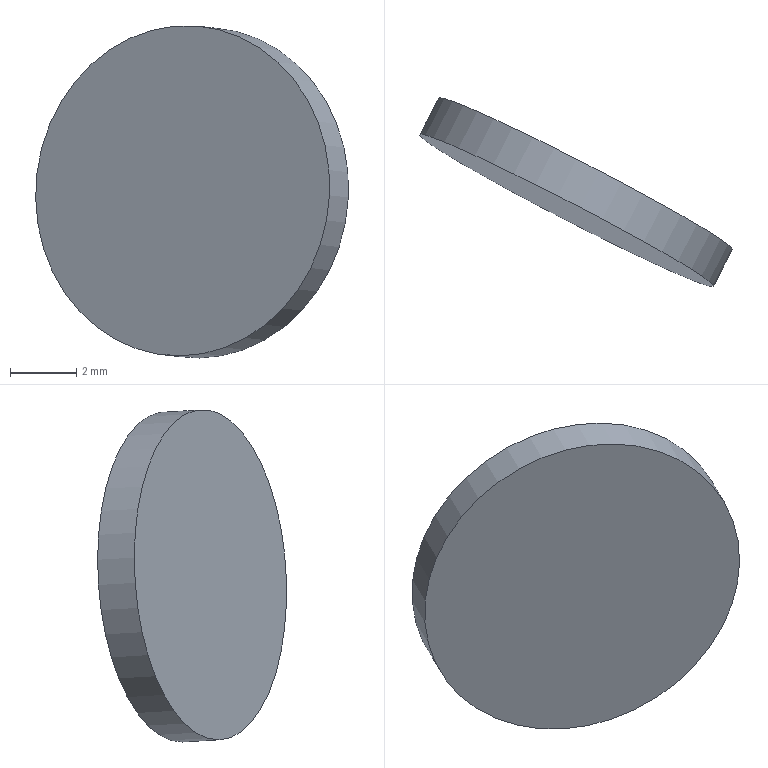Part | STEP file | gslz 2016.10.28-13_id54_x_t | 1 solid | 3 faces | box 9.464 x 5.714 x 10.052 mm | volume 98.175 mm3 | plane 2 | cylinder 1 | commonest cylinder face diameters 10 x1
STEP:
#1=CARTESIAN_POINT('',(0.,0.,0.));
#2=DIRECTION('',(0.,0.,1.));
#3=DIRECTION('',(1.,0.,0.));
#4=AXIS2_PLACEMENT_3D('',#1,#2,#3);
#5=CARTESIAN_POINT('',(875.587,-212.928,-20.691));
#6=VERTEX_POINT('',#5);
#7=CARTESIAN_POINT('',(875.855,-213.36,-25.665));
#8=DIRECTION('',(0.4575,0.8877,-0.05248));
#9=DIRECTION('',(-0.05363,0.08645,0.9948));
#10=AXIS2_PLACEMENT_3D('',#7,#8,#9);
#11=CIRCLE('',#10,5.);
#12=CARTESIAN_POINT('',(876.427,-212.25,-25.731));
#13=DIRECTION('',(-0.4575,-0.8877,0.05248));
#14=DIRECTION('',(0.8889,-0.4581,0.));
#15=AXIS2_PLACEMENT_3D('',#12,#13,#14);
#16=CYLINDRICAL_SURFACE('',#15,5.);
#17=CARTESIAN_POINT('',(7.941,1.25));
#18=DIRECTION('',(-1.,0.));
#19=VECTOR('',#18,1.);
#20=LINE('',#17,#19);
#21=(GEOMETRIC_REPRESENTATION_CONTEXT(2)PARAMETRIC_REPRESENTATION_CONTEXT()REPRESENTATION_CONTEXT('',''));
#22=DEFINITIONAL_REPRESENTATION('',(#20),#21);
#23=PCURVE('',#16,#22);
#24=CARTESIAN_POINT('',(875.855,-213.36,-25.665));
#25=DIRECTION('',(0.4575,0.8877,-0.05248));
#26=DIRECTION('',(-0.8889,0.4581,0.));
#27=AXIS2_PLACEMENT_3D('',#24,#25,#26);
#28=PLANE('',#27);
#29=CARTESIAN_POINT('',(0.,0.));
#30=DIRECTION('',(0.08728,0.9962));
#31=AXIS2_PLACEMENT_2D('',#29,#30);
#32=CIRCLE('',#31,5.);
#33=(GEOMETRIC_REPRESENTATION_CONTEXT(2)PARAMETRIC_REPRESENTATION_CONTEXT()REPRESENTATION_CONTEXT('',''));
#34=DEFINITIONAL_REPRESENTATION('',(#32),#33);
#35=PCURVE('',#28,#34);
#36=SURFACE_CURVE('',#11,(#23,#35),.PCURVE_S1.);
#37=EDGE_CURVE('',#6,#6,#36,.T.);
#38=ORIENTED_EDGE('',*,*,#37,.T.);
#39=CARTESIAN_POINT('',(876.159,-211.818,-20.757));
#40=VERTEX_POINT('',#39);
#41=CARTESIAN_POINT('',(876.159,-211.818,-20.757));
#42=CARTESIAN_POINT('',(875.587,-212.928,-20.691));
#43=B_SPLINE_CURVE_WITH_KNOTS('',1,(#41,#42),.UNSPECIFIED.,.F.,.F.,(2,2),(0.,1.25),.PIECEWISE_BEZIER_KNOTS.);
#44=CARTESIAN_POINT('',(1.658,0.));
#45=DIRECTION('',(0.,1.));
#46=VECTOR('',#45,1.);
#47=LINE('',#44,#46);
#48=(GEOMETRIC_REPRESENTATION_CONTEXT(2)PARAMETRIC_REPRESENTATION_CONTEXT()REPRESENTATION_CONTEXT('',''));
#49=DEFINITIONAL_REPRESENTATION('',(#47),#48);
#50=PCURVE('',#16,#49);
#51=CARTESIAN_POINT('',(7.941,0.));
#52=DIRECTION('',(0.,1.));
#53=VECTOR('',#52,1.);
#54=LINE('',#51,#53);
#55=(GEOMETRIC_REPRESENTATION_CONTEXT(2)PARAMETRIC_REPRESENTATION_CONTEXT()REPRESENTATION_CONTEXT('',''));
#56=DEFINITIONAL_REPRESENTATION('',(#54),#55);
#57=PCURVE('',#16,#56);
#58=SEAM_CURVE('',#43,(#50,#57),.PCURVE_S1.);
#59=EDGE_CURVE('',#40,#6,#58,.T.);
#60=ORIENTED_EDGE('',*,*,#59,.F.);
#61=CARTESIAN_POINT('',(876.427,-212.25,-25.731));
#62=DIRECTION('',(0.4575,0.8877,-0.05248));
#63=DIRECTION('',(-0.05363,0.08645,0.9948));
#64=AXIS2_PLACEMENT_3D('',#61,#62,#63);
#65=CIRCLE('',#64,5.);
#66=CARTESIAN_POINT('',(7.941,0.));
#67=DIRECTION('',(-1.,0.));
#68=VECTOR('',#67,1.);
#69=LINE('',#66,#68);
#70=(GEOMETRIC_REPRESENTATION_CONTEXT(2)PARAMETRIC_REPRESENTATION_CONTEXT()REPRESENTATION_CONTEXT('',''));
#71=DEFINITIONAL_REPRESENTATION('',(#69),#70);
#72=PCURVE('',#16,#71);
#73=CARTESIAN_POINT('',(876.427,-212.25,-25.731));
#74=DIRECTION('',(0.4575,0.8877,-0.05248));
#75=DIRECTION('',(-0.8889,0.4581,0.));
#76=AXIS2_PLACEMENT_3D('',#73,#74,#75);
#77=PLANE('',#76);
#78=CARTESIAN_POINT('',(0.,0.));
#79=DIRECTION('',(0.08728,0.9962));
#80=AXIS2_PLACEMENT_2D('',#78,#79);
#81=CIRCLE('',#80,5.);
#82=(GEOMETRIC_REPRESENTATION_CONTEXT(2)PARAMETRIC_REPRESENTATION_CONTEXT()REPRESENTATION_CONTEXT('',''));
#83=DEFINITIONAL_REPRESENTATION('',(#81),#82);
#84=PCURVE('',#77,#83);
#85=SURFACE_CURVE('',#65,(#72,#84),.PCURVE_S1.);
#86=EDGE_CURVE('',#40,#40,#85,.T.);
#87=ORIENTED_EDGE('',*,*,#86,.F.);
#88=ORIENTED_EDGE('',*,*,#59,.T.);
#89=EDGE_LOOP('',(#38,#60,#87,#88));
#90=FACE_BOUND('',#89,.T.);
#91=ADVANCED_FACE('',(#90),#16,.T.);
#92=ORIENTED_EDGE('',*,*,#86,.T.);
#93=EDGE_LOOP('',(#92));
#94=FACE_BOUND('',#93,.T.);
#95=ADVANCED_FACE('',(#94),#77,.T.);
#96=ORIENTED_EDGE('',*,*,#37,.F.);
#97=EDGE_LOOP('',(#96));
#98=FACE_BOUND('',#97,.T.);
#99=ADVANCED_FACE('',(#98),#28,.F.);
#100=CLOSED_SHELL('',(#91,#95,#99));
#101=MANIFOLD_SOLID_BREP('',#100);
#102=(LENGTH_UNIT()NAMED_UNIT(*)SI_UNIT(.MILLI.,.METRE.));
#103=UNCERTAINTY_MEASURE_WITH_UNIT(LENGTH_MEASURE(0.00001),#102,'','');
#104=(NAMED_UNIT(*)PLANE_ANGLE_UNIT()SI_UNIT($,.RADIAN.));
#105=(NAMED_UNIT(*)SI_UNIT($,.STERADIAN.)SOLID_ANGLE_UNIT());
#106=(GEOMETRIC_REPRESENTATION_CONTEXT(3)GLOBAL_UNCERTAINTY_ASSIGNED_CONTEXT((#103))GLOBAL_UNIT_ASSIGNED_CONTEXT((#102,#104,#105))REPRESENTATION_CONTEXT('',''));
#107=ADVANCED_BREP_SHAPE_REPRESENTATION('',(#4,#101),#106);